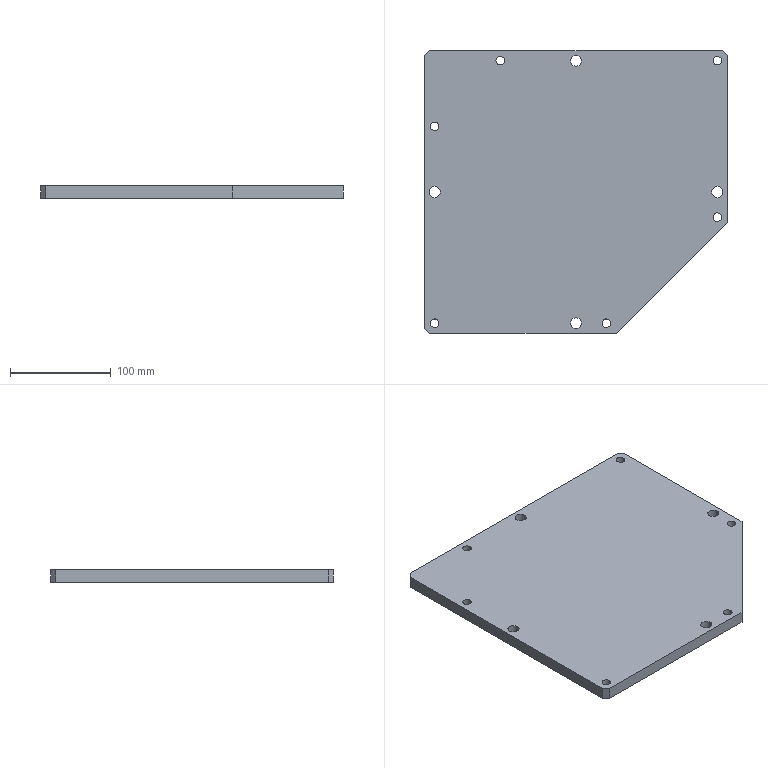Part | STEP file | PN_0002 | 1 solid | 30 faces | box 300 x 280 x 12 mm | volume 926303 mm3 | cylinder 20 | plane 10 | commonest cylinder face diameters 8.5 x12 11 x8